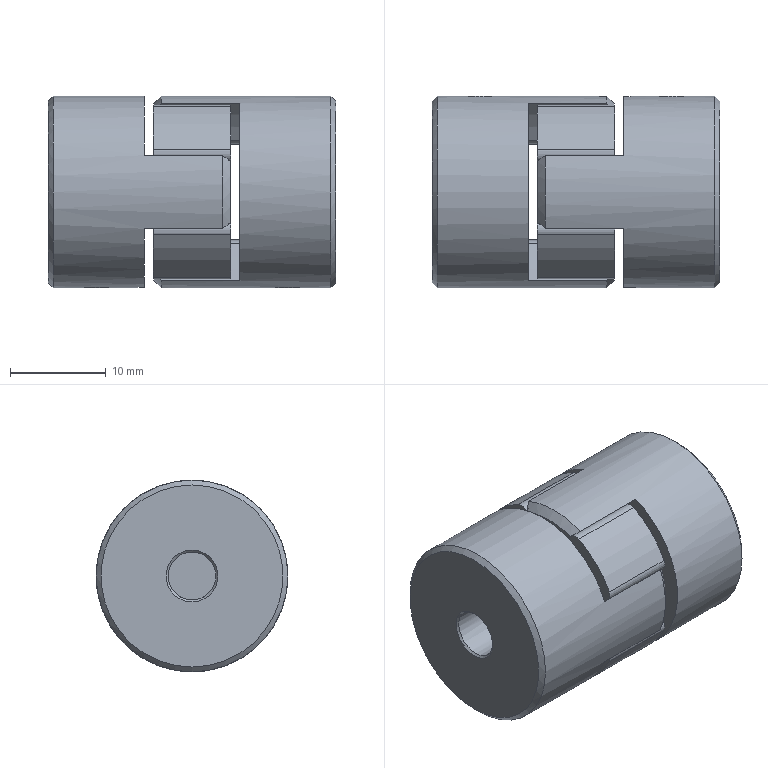Part | STEP file | GCJS20-RD-5-8 | 7 solids | 140 faces | box 30 x 20 x 20 mm | volume 8182 mm3 | plane 66 | cylinder 48 | cone 26 | commonest cylinder face diameters 24 x16 2 x12 20 x6 2.459 x4 3 x4 9.5 x4